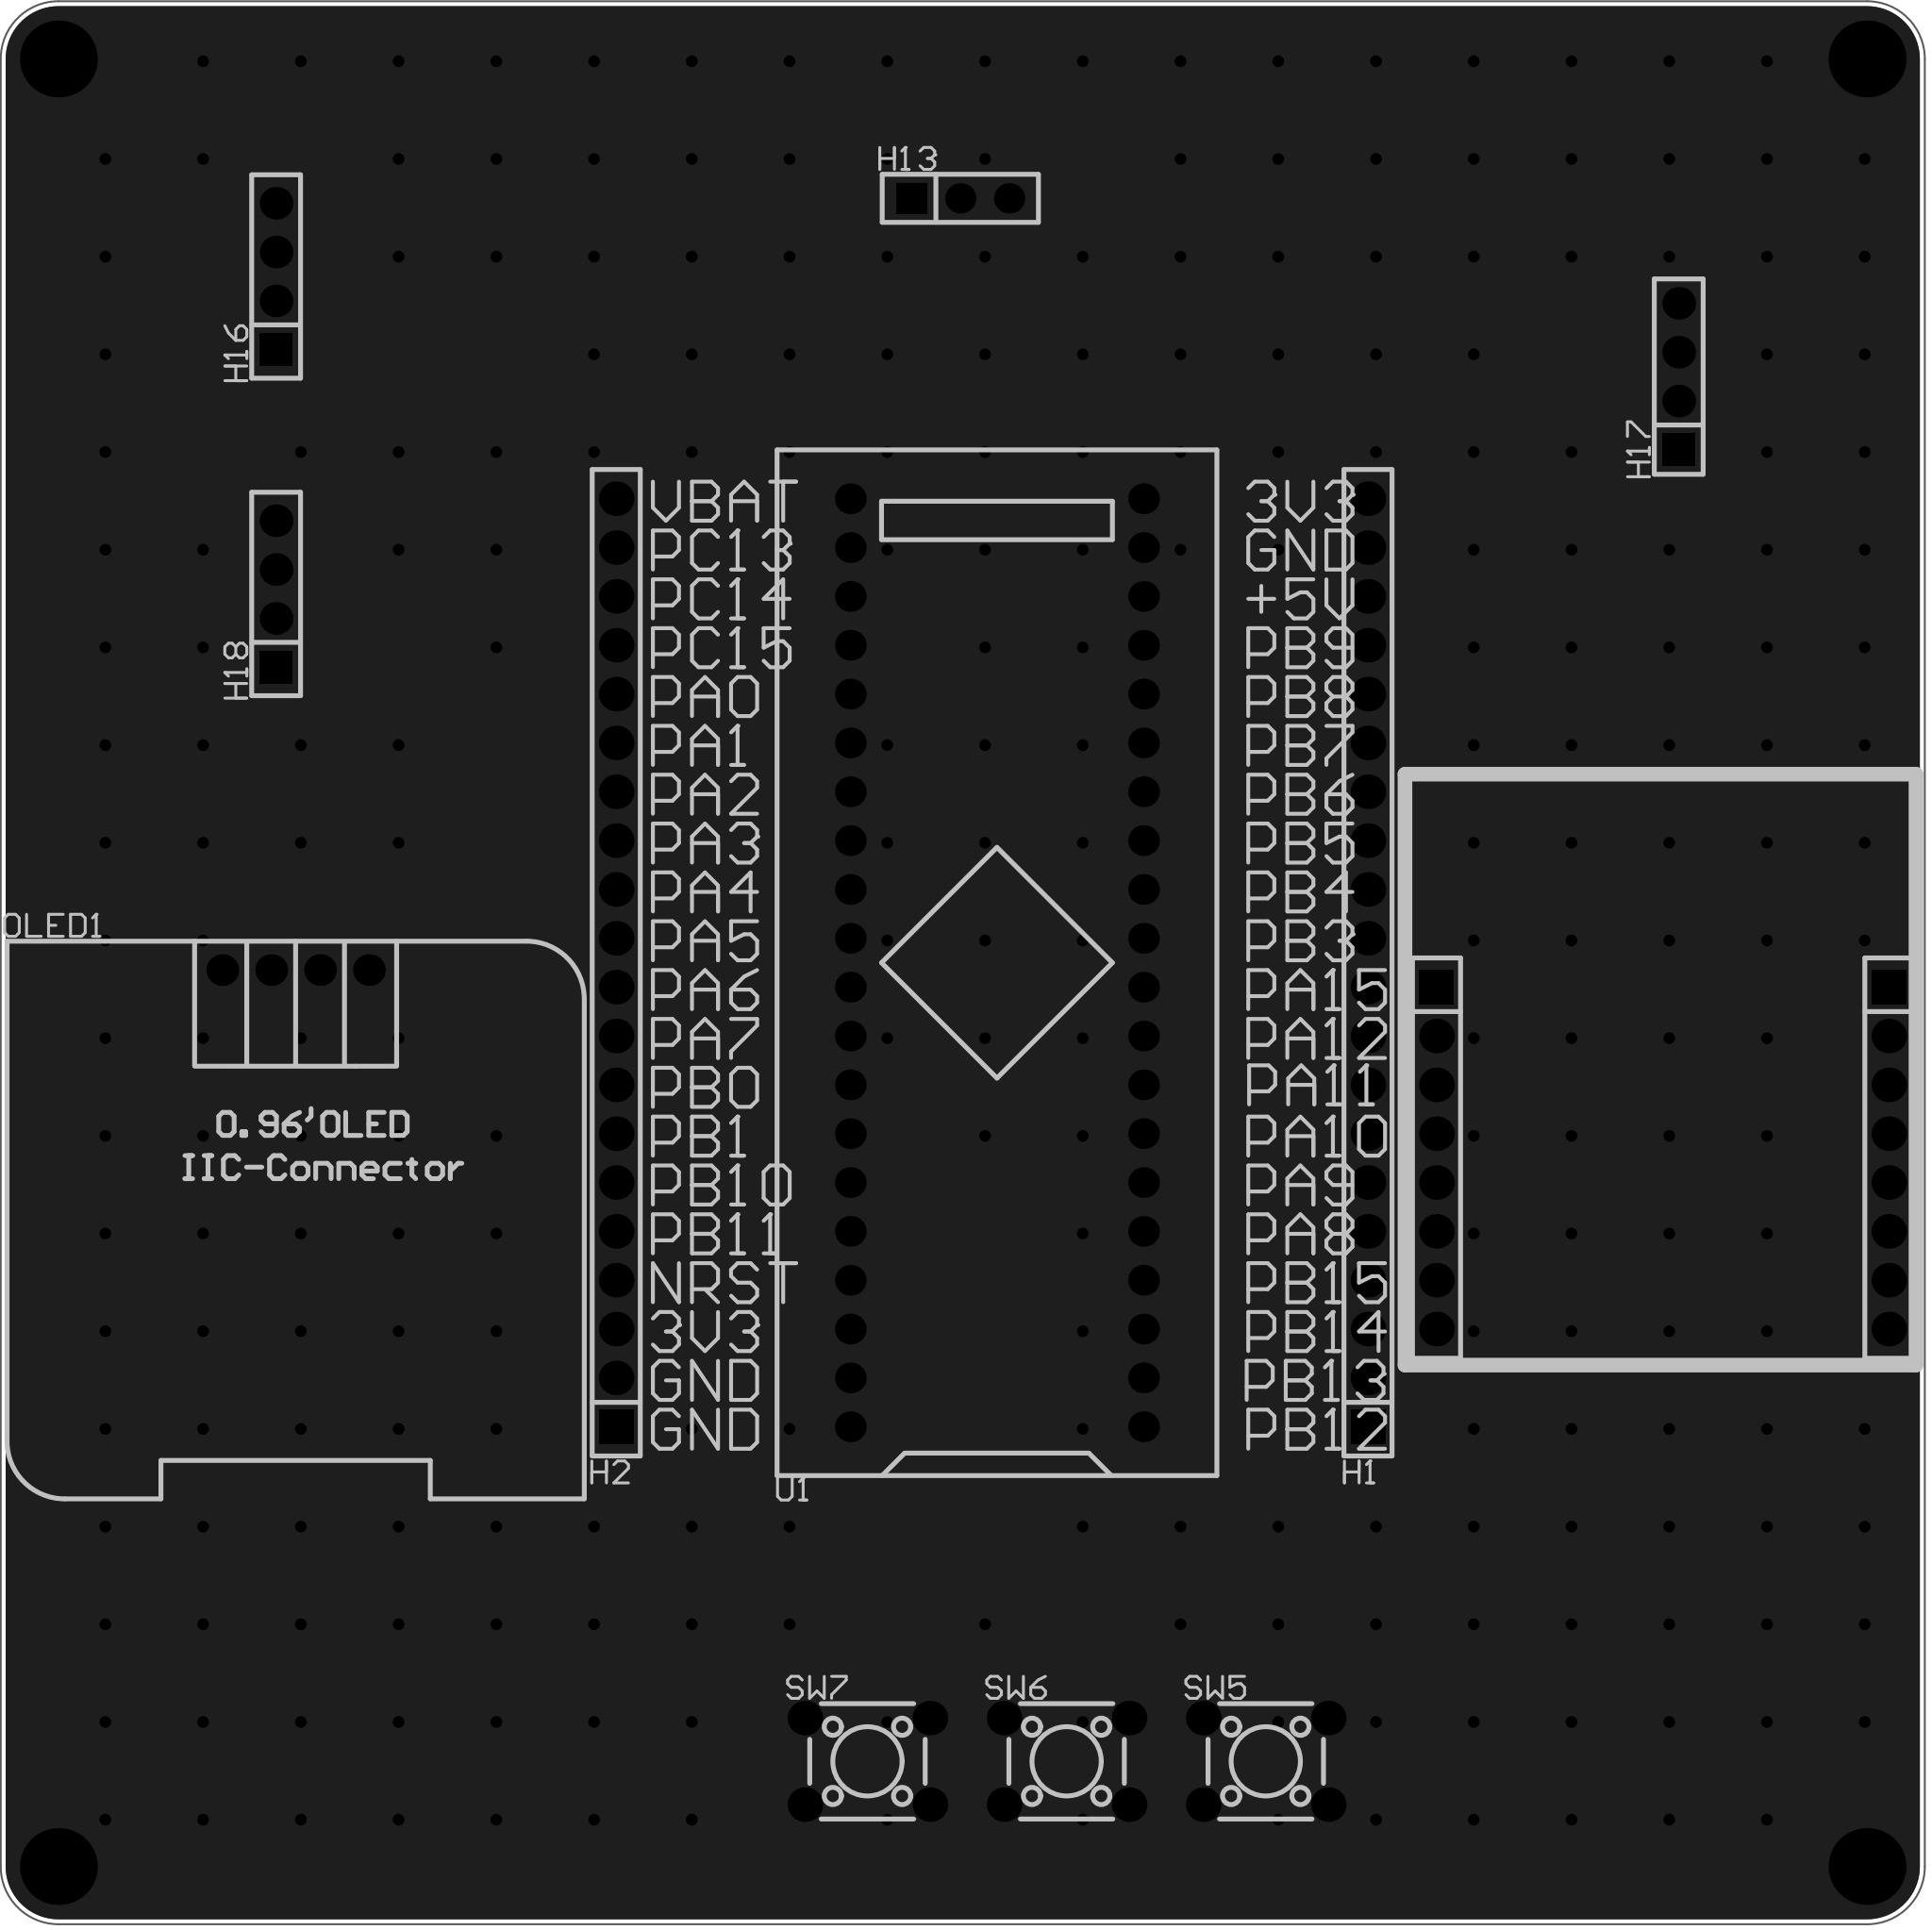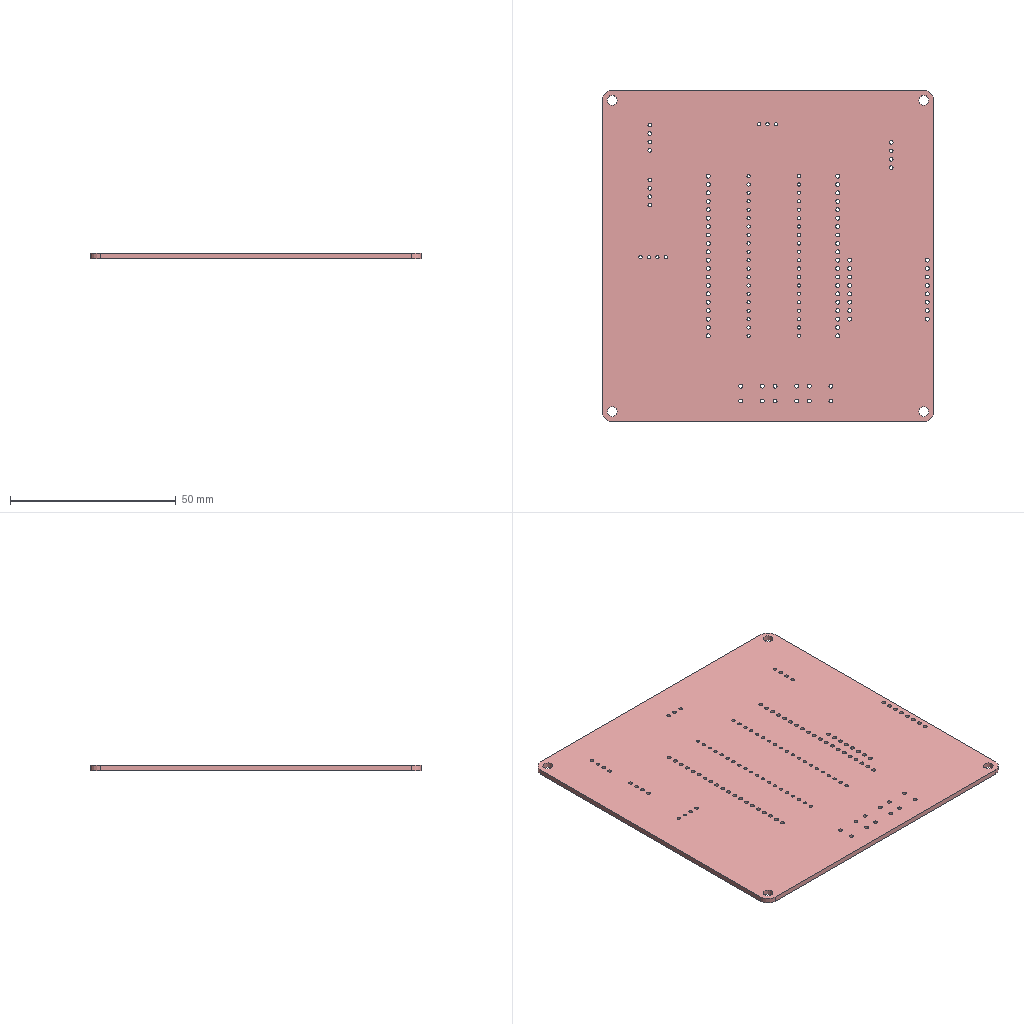Circuit board layout | Altium Designer | box 100 x 100 x 1.6 mm
Layer stack:
# Altium Designer layer stack of  (unit mm; dielectric type: 0 none, 1 core, 2 prepreg, 3 surface material)
index,name,kind,layer,copper_thickness_mm,dielectric_type,dielectric_thickness_mm,dielectric_material,dielectric_constant
0,Top Paste Mask Layer,other,,,,,,
1,Top Silkscreen Layer,other,,,,,,
2,Top Solder Mask Layer,dielectric,,,3,0.01,,3.3
3,Top Layer,copper,Top Layer,0.035,,,,
4,Dielectric1,dielectric,,,3,1.51,FR4,4.5
5,Bottom Layer,copper,Bottom Layer,0.035,,,,
6,Bottom Solder Mask Layer,dielectric,,,3,0.01,,3.3
7,Bottom Silkscreen Layer,other,,,,,,
8,Bottom Paste Mask Layer,other,,,,,,
# drill layer pairs: low layer,high layer
drill_pair,Top Layer,Bottom Layer
Part placement:
Designator,Comment,Layer,Footprint,Center-X(mm),Center-Y(mm),Rotation
U1,STM32F103C8T6-Card,TopLayer,CONN-TH_L53.3-W22.9_STM32F103C8T6-CARD,132.334,128.905,90
H16,,TopLayer,HDR-TH_4P-P2.54-V-F,94.869,164.592,90
H17,,TopLayer,HDR-TH_4P-P2.54-V-M,167.767,159.385,90
H18,,TopLayer,HDR-TH_4P-P2.54-V-F,94.869,148.082,90
H1,,TopLayer,HDR-TH_20P-P2.54-V-F,151.617,128.905,90
H2,,TopLayer,HDR-TH_20P-P2.54-V-F,112.546,128.905,90
OLED1,,TopLayer,0.96OLED_4P,95.885,128.524,0
H13,,TopLayer,HDR-TH_3P-P2.54-V-F,130.429,168.656,0
SW5,,TopLayer,SW-TH_4P-L6.0-W6.0-P4.50-LS6.5,146.304,87.376,0
SW6,,TopLayer,SW-TH_4P-L6.0-W6.0-P4.50-LS6.5,135.953,87.376,0
SW7,,TopLayer,SW-TH_4P-L6.0-W6.0-P4.50-LS6.5,125.603,87.376,0
H14,,TopLayer,HDR-TH_8P-P2.54-V-F-1,155.179,118.745,270
H15,,TopLayer,HDR-TH_8P-P2.54-V-F-1,178.689,118.745,270
Pad and via stacks:
# Altium Designer via and pad stacks of  (unit mm). Each distinct definition once, with the count of objects using it.
# via: kind,start_layer,end_layer,hole_mm,diameter_mm,mode(0 simple;1 top-mid-bottom;2 full stack),diameter_per_layer,count,example_net
# pad: kind,layer,hole_mm,hole_type(0 round;1 square;2 slot),plating,top_size,top_shape(1 round;2 rect;3 octagon;9 rounded rect),mid_size,bottom_size,mode,footprint,size_per_layer,count,example
pad,Multi-Layer,3,0,plated,4x4,1,4x4,4x4,0,,,4,1
pad,Multi-Layer,1,0,plated,1.6x1.6,1,1.6x1.6,1.6x1.6,0,CONN-TH_L53.3-W22.9_STM32F103C8T6-CARD,,40,U1.1
pad,Multi-Layer,1.1,0,plated,1.7x1.7,2,1.7x1.7,1.7x1.7,0,HDR-TH_4P-P2.54-V-F,,2,H16.1
pad,Multi-Layer,1.1,0,plated,1.7x1.7,1,1.7x1.7,1.7x1.7,0,HDR-TH_4P-P2.54-V-F,,6,H16.2
pad,Multi-Layer,1.1,0,plated,1.7x1.7,2,1.7x1.7,1.7x1.7,0,HDR-TH_4P-P2.54-V-M,,1,H17.1
pad,Multi-Layer,1.1,0,plated,1.7x1.7,1,1.7x1.7,1.7x1.7,0,HDR-TH_4P-P2.54-V-M,,3,H17.2
pad,Multi-Layer,1.2,0,plated,1.8x1.8,2,1.8x1.8,1.8x1.8,0,HDR-TH_20P-P2.54-V-F,,2,H1.1
pad,Multi-Layer,1.2,0,plated,1.8x1.8,1,1.8x1.8,1.8x1.8,0,HDR-TH_20P-P2.54-V-F,,38,H1.2
pad,Multi-Layer,1,0,plated,1.65x1.65,1,1.65x1.65,1.65x1.65,0,0.96OLED_4P,,4,OLED1.4
pad,Multi-Layer,1.02,0,plated,1.575x1.575,1,1.575x1.575,1.575x1.575,0,HDR-TH_3P-P2.54-V-F,,2,H13.3
pad,Multi-Layer,1.02,0,plated,1.575x1.575,2,1.575x1.575,1.575x1.575,0,HDR-TH_3P-P2.54-V-F,,1,H13.1
pad,Multi-Layer,1.2,0,plated,1.8x1.8,1,1.8x1.8,1.8x1.8,0,SW-TH_4P-L6.0-W6.0-P4.50-LS6.5,,12,SW5.1
pad,Multi-Layer,1.2,0,plated,1.8x1.8,2,1.8x1.8,1.8x1.8,0,HDR-TH_8P-P2.54-V-F-1,,2,H14.1
pad,Multi-Layer,1.2,0,plated,1.8x1.8,1,1.8x1.8,1.8x1.8,0,HDR-TH_8P-P2.54-V-F-1,,14,H14.2
via,Top Layer,Bottom Layer,0.3048,0.61,0,,259,GND
Copper pours:
name,layer,net,type(0 solid;1 hatched;2 none)
Bottom Layer-GND,Bottom Layer,GND,0
Top Layer-GND,Top Layer,GND,0